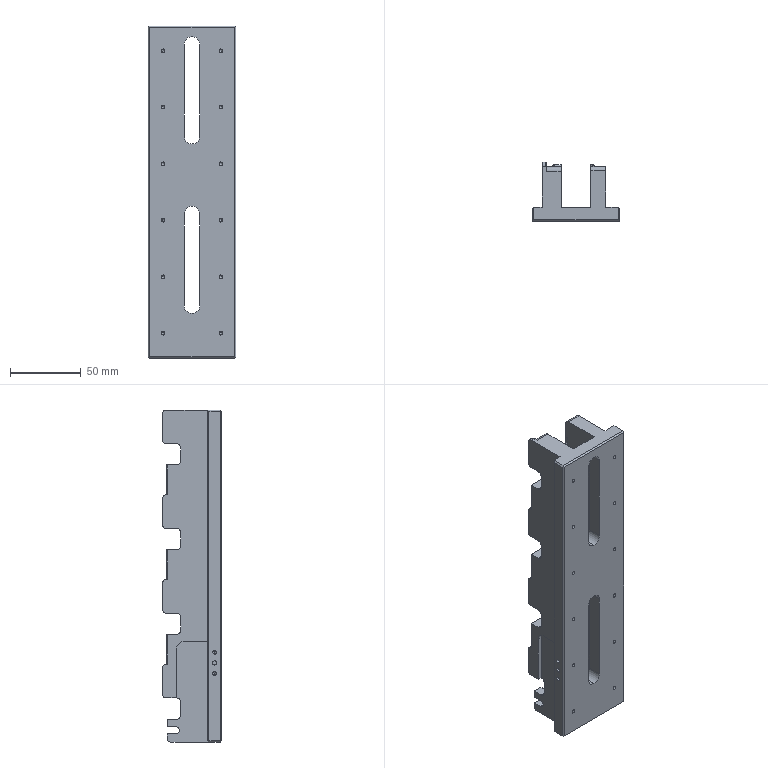Part | STEP file | 01-02 loading sliding plate | 1 solid | 331 faces | box 62 x 42 x 235 mm | volume 266877 mm3 | plane 138 | cylinder 137 | cone 32 | spline 16 | torus 8 | commonest cylinder face diameters 2.5 x32 6 x25 1.6 x24 1 x20 2 x16 4 x8